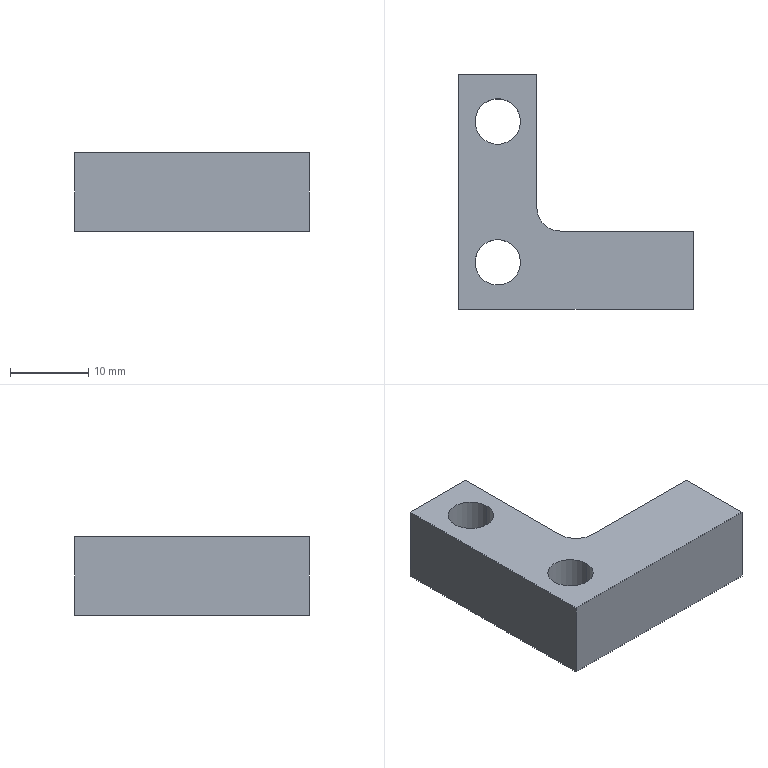Part | SolidWorks | features BaseBody 1 | 1 solid | 13 faces | box 30 x 30 x 10 mm | volume 4491 mm3 | plane 8 | cylinder 5 | commonest cylinder face diameters 5.8 x4 6 x1
STEP:
#1=CARTESIAN_POINT('',(-12.9,9.,0.));
#2=VERTEX_POINT('',#1);
#3=CARTESIAN_POINT('',(-12.9,9.,10.));
#4=VERTEX_POINT('',#3);
#5=CARTESIAN_POINT('',(-12.9,9.,10.));
#6=DIRECTION('',(0.,0.,1.));
#7=VECTOR('',#6,1000.);
#8=LINE('',#5,#7);
#9=EDGE_CURVE('',#2,#4,#8,.T.);
#10=ORIENTED_EDGE('',*,*,#9,.F.);
#11=CARTESIAN_POINT('',(-7.1,9.,0.));
#12=VERTEX_POINT('',#11);
#13=CARTESIAN_POINT('',(-10.,9.,0.));
#14=DIRECTION('',(0.,0.,1.));
#15=DIRECTION('',(1.,0.,0.));
#16=AXIS2_PLACEMENT_3D('',#13,#14,#15);
#17=CIRCLE('',#16,2.9);
#18=EDGE_CURVE('',#12,#2,#17,.T.);
#19=ORIENTED_EDGE('',*,*,#18,.F.);
#20=CARTESIAN_POINT('',(-7.1,9.,10.));
#21=VERTEX_POINT('',#20);
#22=CARTESIAN_POINT('',(-7.1,9.,10.));
#23=DIRECTION('',(0.,0.,1.));
#24=VECTOR('',#23,1000.);
#25=LINE('',#22,#24);
#26=EDGE_CURVE('',#12,#21,#25,.T.);
#27=ORIENTED_EDGE('',*,*,#26,.T.);
#28=CARTESIAN_POINT('',(-10.,9.,10.));
#29=DIRECTION('',(0.,0.,1.));
#30=DIRECTION('',(1.,0.,0.));
#31=AXIS2_PLACEMENT_3D('',#28,#29,#30);
#32=CIRCLE('',#31,2.9);
#33=EDGE_CURVE('',#21,#4,#32,.T.);
#34=ORIENTED_EDGE('',*,*,#33,.T.);
#35=EDGE_LOOP('',(#10,#19,#27,#34));
#36=FACE_OUTER_BOUND('',#35,.T.);
#37=CARTESIAN_POINT('',(-10.,9.,10.));
#38=DIRECTION('',(0.,0.,1.));
#39=DIRECTION('',(1.,0.,0.));
#40=AXIS2_PLACEMENT_3D('',#37,#38,#39);
#41=CYLINDRICAL_SURFACE('',#40,2.9);
#42=ADVANCED_FACE('',(#36),#41,.F.);
#43=CARTESIAN_POINT('',(-12.9,-9.,0.));
#44=VERTEX_POINT('',#43);
#45=CARTESIAN_POINT('',(-12.9,-9.,10.));
#46=VERTEX_POINT('',#45);
#47=CARTESIAN_POINT('',(-12.9,-9.,10.));
#48=DIRECTION('',(0.,0.,1.));
#49=VECTOR('',#48,1000.);
#50=LINE('',#47,#49);
#51=EDGE_CURVE('',#44,#46,#50,.T.);
#52=ORIENTED_EDGE('',*,*,#51,.F.);
#53=CARTESIAN_POINT('',(-7.1,-9.,0.));
#54=VERTEX_POINT('',#53);
#55=CARTESIAN_POINT('',(-10.,-9.,0.));
#56=DIRECTION('',(0.,0.,1.));
#57=DIRECTION('',(1.,0.,0.));
#58=AXIS2_PLACEMENT_3D('',#55,#56,#57);
#59=CIRCLE('',#58,2.9);
#60=EDGE_CURVE('',#54,#44,#59,.T.);
#61=ORIENTED_EDGE('',*,*,#60,.F.);
#62=CARTESIAN_POINT('',(-7.1,-9.,10.));
#63=VERTEX_POINT('',#62);
#64=CARTESIAN_POINT('',(-7.1,-9.,10.));
#65=DIRECTION('',(0.,0.,1.));
#66=VECTOR('',#65,1000.);
#67=LINE('',#64,#66);
#68=EDGE_CURVE('',#54,#63,#67,.T.);
#69=ORIENTED_EDGE('',*,*,#68,.T.);
#70=CARTESIAN_POINT('',(-10.,-9.,10.));
#71=DIRECTION('',(0.,0.,1.));
#72=DIRECTION('',(1.,0.,0.));
#73=AXIS2_PLACEMENT_3D('',#70,#71,#72);
#74=CIRCLE('',#73,2.9);
#75=EDGE_CURVE('',#63,#46,#74,.T.);
#76=ORIENTED_EDGE('',*,*,#75,.T.);
#77=EDGE_LOOP('',(#52,#61,#69,#76));
#78=FACE_OUTER_BOUND('',#77,.T.);
#79=CARTESIAN_POINT('',(-10.,-9.,10.));
#80=DIRECTION('',(0.,0.,1.));
#81=DIRECTION('',(1.,0.,0.));
#82=AXIS2_PLACEMENT_3D('',#79,#80,#81);
#83=CYLINDRICAL_SURFACE('',#82,2.9);
#84=ADVANCED_FACE('',(#78),#83,.F.);
#85=CARTESIAN_POINT('',(-5.,-2.,0.));
#86=VERTEX_POINT('',#85);
#87=CARTESIAN_POINT('',(-2.,-5.,0.));
#88=VERTEX_POINT('',#87);
#89=CARTESIAN_POINT('',(-2.,-2.,0.));
#90=DIRECTION('',(0.,0.,1.));
#91=DIRECTION('',(1.,0.,0.));
#92=AXIS2_PLACEMENT_3D('',#89,#90,#91);
#93=CIRCLE('',#92,3.);
#94=EDGE_CURVE('',#86,#88,#93,.T.);
#95=ORIENTED_EDGE('',*,*,#94,.F.);
#96=CARTESIAN_POINT('',(-5.,-2.,10.));
#97=VERTEX_POINT('',#96);
#98=CARTESIAN_POINT('',(-5.,-2.,0.));
#99=DIRECTION('',(0.,0.,-1.));
#100=VECTOR('',#99,1000.);
#101=LINE('',#98,#100);
#102=EDGE_CURVE('',#97,#86,#101,.T.);
#103=ORIENTED_EDGE('',*,*,#102,.F.);
#104=CARTESIAN_POINT('',(-2.,-5.,10.));
#105=VERTEX_POINT('',#104);
#106=CARTESIAN_POINT('',(-2.,-2.,10.));
#107=DIRECTION('',(0.,0.,-1.));
#108=DIRECTION('',(1.,0.,0.));
#109=AXIS2_PLACEMENT_3D('',#106,#107,#108);
#110=CIRCLE('',#109,3.);
#111=EDGE_CURVE('',#105,#97,#110,.T.);
#112=ORIENTED_EDGE('',*,*,#111,.F.);
#113=CARTESIAN_POINT('',(-2.,-5.,10.));
#114=DIRECTION('',(0.,0.,1.));
#115=VECTOR('',#114,1000.);
#116=LINE('',#113,#115);
#117=EDGE_CURVE('',#88,#105,#116,.T.);
#118=ORIENTED_EDGE('',*,*,#117,.F.);
#119=EDGE_LOOP('',(#95,#103,#112,#118));
#120=FACE_OUTER_BOUND('',#119,.T.);
#121=CARTESIAN_POINT('',(-2.,-2.,-0.001));
#122=DIRECTION('',(0.,0.,-1.));
#123=DIRECTION('',(-1.,0.,0.));
#124=AXIS2_PLACEMENT_3D('',#121,#122,#123);
#125=CYLINDRICAL_SURFACE('',#124,3.);
#126=ADVANCED_FACE('',(#120),#125,.F.);
#127=CARTESIAN_POINT('',(-5.,15.,10.));
#128=VERTEX_POINT('',#127);
#129=CARTESIAN_POINT('',(-5.,15.,10.));
#130=DIRECTION('',(0.,-1.,0.));
#131=VECTOR('',#130,1000.);
#132=LINE('',#129,#131);
#133=EDGE_CURVE('',#128,#97,#132,.T.);
#134=ORIENTED_EDGE('',*,*,#133,.T.);
#135=ORIENTED_EDGE('',*,*,#102,.T.);
#136=CARTESIAN_POINT('',(-5.,15.,0.));
#137=VERTEX_POINT('',#136);
#138=CARTESIAN_POINT('',(-5.,15.,0.));
#139=DIRECTION('',(0.,1.,0.));
#140=VECTOR('',#139,1000.);
#141=LINE('',#138,#140);
#142=EDGE_CURVE('',#86,#137,#141,.T.);
#143=ORIENTED_EDGE('',*,*,#142,.T.);
#144=CARTESIAN_POINT('',(-5.,15.,-0.001));
#145=DIRECTION('',(0.,0.,1.));
#146=VECTOR('',#145,1000.);
#147=LINE('',#144,#146);
#148=EDGE_CURVE('',#137,#128,#147,.T.);
#149=ORIENTED_EDGE('',*,*,#148,.T.);
#150=EDGE_LOOP('',(#134,#135,#143,#149));
#151=FACE_OUTER_BOUND('',#150,.T.);
#152=CARTESIAN_POINT('',(-5.,15.,-0.001));
#153=DIRECTION('',(-1.,0.,0.));
#154=DIRECTION('',(0.,1.,0.));
#155=AXIS2_PLACEMENT_3D('',#152,#153,#154);
#156=PLANE('',#155);
#157=ADVANCED_FACE('',(#151),#156,.F.);
#158=CARTESIAN_POINT('',(15.,-5.,0.));
#159=VERTEX_POINT('',#158);
#160=CARTESIAN_POINT('',(15.,-5.,0.));
#161=DIRECTION('',(-1.,0.,0.));
#162=VECTOR('',#161,1000.);
#163=LINE('',#160,#162);
#164=EDGE_CURVE('',#159,#88,#163,.T.);
#165=ORIENTED_EDGE('',*,*,#164,.T.);
#166=ORIENTED_EDGE('',*,*,#117,.T.);
#167=CARTESIAN_POINT('',(15.,-5.,10.));
#168=VERTEX_POINT('',#167);
#169=CARTESIAN_POINT('',(15.,-5.,10.));
#170=DIRECTION('',(1.,0.,0.));
#171=VECTOR('',#170,1000.);
#172=LINE('',#169,#171);
#173=EDGE_CURVE('',#105,#168,#172,.T.);
#174=ORIENTED_EDGE('',*,*,#173,.T.);
#175=CARTESIAN_POINT('',(15.,-5.,-0.001));
#176=DIRECTION('',(0.,0.,1.));
#177=VECTOR('',#176,1000.);
#178=LINE('',#175,#177);
#179=EDGE_CURVE('',#159,#168,#178,.T.);
#180=ORIENTED_EDGE('',*,*,#179,.F.);
#181=EDGE_LOOP('',(#165,#166,#174,#180));
#182=FACE_OUTER_BOUND('',#181,.T.);
#183=CARTESIAN_POINT('',(15.,-5.,-0.001));
#184=DIRECTION('',(0.,-1.,0.));
#185=DIRECTION('',(0.,0.,-1.));
#186=AXIS2_PLACEMENT_3D('',#183,#184,#185);
#187=PLANE('',#186);
#188=ADVANCED_FACE('',(#182),#187,.F.);
#189=ORIENTED_EDGE('',*,*,#60,.T.);
#190=CARTESIAN_POINT('',(-10.,-9.,0.));
#191=DIRECTION('',(0.,0.,1.));
#192=DIRECTION('',(1.,0.,0.));
#193=AXIS2_PLACEMENT_3D('',#190,#191,#192);
#194=CIRCLE('',#193,2.9);
#195=EDGE_CURVE('',#44,#54,#194,.T.);
#196=ORIENTED_EDGE('',*,*,#195,.T.);
#197=EDGE_LOOP('',(#189,#196));
#198=FACE_BOUND('',#197,.T.);
#199=ORIENTED_EDGE('',*,*,#18,.T.);
#200=CARTESIAN_POINT('',(-10.,9.,0.));
#201=DIRECTION('',(0.,0.,1.));
#202=DIRECTION('',(1.,0.,0.));
#203=AXIS2_PLACEMENT_3D('',#200,#201,#202);
#204=CIRCLE('',#203,2.9);
#205=EDGE_CURVE('',#2,#12,#204,.T.);
#206=ORIENTED_EDGE('',*,*,#205,.T.);
#207=EDGE_LOOP('',(#199,#206));
#208=FACE_BOUND('',#207,.T.);
#209=ORIENTED_EDGE('',*,*,#142,.F.);
#210=ORIENTED_EDGE('',*,*,#94,.T.);
#211=ORIENTED_EDGE('',*,*,#164,.F.);
#212=CARTESIAN_POINT('',(15.,-15.,0.));
#213=VERTEX_POINT('',#212);
#214=CARTESIAN_POINT('',(15.,-15.,0.));
#215=DIRECTION('',(0.,1.,0.));
#216=VECTOR('',#215,1000.);
#217=LINE('',#214,#216);
#218=EDGE_CURVE('',#213,#159,#217,.T.);
#219=ORIENTED_EDGE('',*,*,#218,.F.);
#220=CARTESIAN_POINT('',(-15.,-15.,0.));
#221=VERTEX_POINT('',#220);
#222=CARTESIAN_POINT('',(15.,-15.,0.));
#223=DIRECTION('',(1.,0.,0.));
#224=VECTOR('',#223,1000.);
#225=LINE('',#222,#224);
#226=EDGE_CURVE('',#221,#213,#225,.T.);
#227=ORIENTED_EDGE('',*,*,#226,.F.);
#228=CARTESIAN_POINT('',(-15.,15.,0.));
#229=VERTEX_POINT('',#228);
#230=CARTESIAN_POINT('',(-15.,-15.,0.));
#231=DIRECTION('',(0.,-1.,0.));
#232=VECTOR('',#231,1000.);
#233=LINE('',#230,#232);
#234=EDGE_CURVE('',#229,#221,#233,.T.);
#235=ORIENTED_EDGE('',*,*,#234,.F.);
#236=CARTESIAN_POINT('',(15.,15.,0.));
#237=DIRECTION('',(-1.,0.,0.));
#238=VECTOR('',#237,1000.);
#239=LINE('',#236,#238);
#240=EDGE_CURVE('',#137,#229,#239,.T.);
#241=ORIENTED_EDGE('',*,*,#240,.F.);
#242=EDGE_LOOP('',(#209,#210,#211,#219,#227,#235,#241));
#243=FACE_OUTER_BOUND('',#242,.T.);
#244=CARTESIAN_POINT('',(0.,0.,0.));
#245=DIRECTION('',(0.,0.,1.));
#246=DIRECTION('',(1.,0.,0.));
#247=AXIS2_PLACEMENT_3D('',#244,#245,#246);
#248=PLANE('',#247);
#249=ADVANCED_FACE('',(#198,#208,#243),#248,.F.);
#250=ORIENTED_EDGE('',*,*,#75,.F.);
#251=CARTESIAN_POINT('',(-10.,-9.,10.));
#252=DIRECTION('',(0.,0.,1.));
#253=DIRECTION('',(1.,0.,0.));
#254=AXIS2_PLACEMENT_3D('',#251,#252,#253);
#255=CIRCLE('',#254,2.9);
#256=EDGE_CURVE('',#46,#63,#255,.T.);
#257=ORIENTED_EDGE('',*,*,#256,.F.);
#258=EDGE_LOOP('',(#250,#257));
#259=FACE_BOUND('',#258,.T.);
#260=ORIENTED_EDGE('',*,*,#33,.F.);
#261=CARTESIAN_POINT('',(-10.,9.,10.));
#262=DIRECTION('',(0.,0.,1.));
#263=DIRECTION('',(1.,0.,0.));
#264=AXIS2_PLACEMENT_3D('',#261,#262,#263);
#265=CIRCLE('',#264,2.9);
#266=EDGE_CURVE('',#4,#21,#265,.T.);
#267=ORIENTED_EDGE('',*,*,#266,.F.);
#268=EDGE_LOOP('',(#260,#267));
#269=FACE_BOUND('',#268,.T.);
#270=ORIENTED_EDGE('',*,*,#173,.F.);
#271=ORIENTED_EDGE('',*,*,#111,.T.);
#272=ORIENTED_EDGE('',*,*,#133,.F.);
#273=CARTESIAN_POINT('',(-15.,15.,10.));
#274=VERTEX_POINT('',#273);
#275=CARTESIAN_POINT('',(15.,15.,10.));
#276=DIRECTION('',(-1.,0.,0.));
#277=VECTOR('',#276,1000.);
#278=LINE('',#275,#277);
#279=EDGE_CURVE('',#128,#274,#278,.T.);
#280=ORIENTED_EDGE('',*,*,#279,.T.);
#281=CARTESIAN_POINT('',(-15.,-15.,10.));
#282=VERTEX_POINT('',#281);
#283=CARTESIAN_POINT('',(-15.,-15.,10.));
#284=DIRECTION('',(0.,-1.,0.));
#285=VECTOR('',#284,1000.);
#286=LINE('',#283,#285);
#287=EDGE_CURVE('',#274,#282,#286,.T.);
#288=ORIENTED_EDGE('',*,*,#287,.T.);
#289=CARTESIAN_POINT('',(15.,-15.,10.));
#290=VERTEX_POINT('',#289);
#291=CARTESIAN_POINT('',(15.,-15.,10.));
#292=DIRECTION('',(1.,0.,0.));
#293=VECTOR('',#292,1000.);
#294=LINE('',#291,#293);
#295=EDGE_CURVE('',#282,#290,#294,.T.);
#296=ORIENTED_EDGE('',*,*,#295,.T.);
#297=CARTESIAN_POINT('',(15.,-15.,10.));
#298=DIRECTION('',(0.,1.,0.));
#299=VECTOR('',#298,1000.);
#300=LINE('',#297,#299);
#301=EDGE_CURVE('',#290,#168,#300,.T.);
#302=ORIENTED_EDGE('',*,*,#301,.T.);
#303=EDGE_LOOP('',(#270,#271,#272,#280,#288,#296,#302));
#304=FACE_OUTER_BOUND('',#303,.T.);
#305=CARTESIAN_POINT('',(0.,0.,10.));
#306=DIRECTION('',(0.,0.,1.));
#307=DIRECTION('',(1.,0.,0.));
#308=AXIS2_PLACEMENT_3D('',#305,#306,#307);
#309=PLANE('',#308);
#310=ADVANCED_FACE('',(#259,#269,#304),#309,.T.);
#311=ORIENTED_EDGE('',*,*,#279,.F.);
#312=ORIENTED_EDGE('',*,*,#148,.F.);
#313=ORIENTED_EDGE('',*,*,#240,.T.);
#314=CARTESIAN_POINT('',(-15.,15.,10.));
#315=DIRECTION('',(0.,0.,-1.));
#316=VECTOR('',#315,1000.);
#317=LINE('',#314,#316);
#318=EDGE_CURVE('',#274,#229,#317,.T.);
#319=ORIENTED_EDGE('',*,*,#318,.F.);
#320=EDGE_LOOP('',(#311,#312,#313,#319));
#321=FACE_OUTER_BOUND('',#320,.T.);
#322=CARTESIAN_POINT('',(15.,15.,10.));
#323=DIRECTION('',(0.,-1.,0.));
#324=DIRECTION('',(0.,0.,-1.));
#325=AXIS2_PLACEMENT_3D('',#322,#323,#324);
#326=PLANE('',#325);
#327=ADVANCED_FACE('',(#321),#326,.F.);
#328=ORIENTED_EDGE('',*,*,#218,.T.);
#329=ORIENTED_EDGE('',*,*,#179,.T.);
#330=ORIENTED_EDGE('',*,*,#301,.F.);
#331=CARTESIAN_POINT('',(15.,-15.,10.));
#332=DIRECTION('',(0.,0.,-1.));
#333=VECTOR('',#332,1000.);
#334=LINE('',#331,#333);
#335=EDGE_CURVE('',#290,#213,#334,.T.);
#336=ORIENTED_EDGE('',*,*,#335,.T.);
#337=EDGE_LOOP('',(#328,#329,#330,#336));
#338=FACE_OUTER_BOUND('',#337,.T.);
#339=CARTESIAN_POINT('',(15.,-15.,10.));
#340=DIRECTION('',(-1.,0.,0.));
#341=DIRECTION('',(0.,0.,1.));
#342=AXIS2_PLACEMENT_3D('',#339,#340,#341);
#343=PLANE('',#342);
#344=ADVANCED_FACE('',(#338),#343,.F.);
#345=ORIENTED_EDGE('',*,*,#226,.T.);
#346=ORIENTED_EDGE('',*,*,#335,.F.);
#347=ORIENTED_EDGE('',*,*,#295,.F.);
#348=CARTESIAN_POINT('',(-15.,-15.,10.));
#349=DIRECTION('',(0.,0.,-1.));
#350=VECTOR('',#349,1000.);
#351=LINE('',#348,#350);
#352=EDGE_CURVE('',#282,#221,#351,.T.);
#353=ORIENTED_EDGE('',*,*,#352,.T.);
#354=EDGE_LOOP('',(#345,#346,#347,#353));
#355=FACE_OUTER_BOUND('',#354,.T.);
#356=CARTESIAN_POINT('',(15.,-15.,10.));
#357=DIRECTION('',(0.,1.,0.));
#358=DIRECTION('',(1.,0.,0.));
#359=AXIS2_PLACEMENT_3D('',#356,#357,#358);
#360=PLANE('',#359);
#361=ADVANCED_FACE('',(#355),#360,.F.);
#362=ORIENTED_EDGE('',*,*,#234,.T.);
#363=ORIENTED_EDGE('',*,*,#352,.F.);
#364=ORIENTED_EDGE('',*,*,#287,.F.);
#365=ORIENTED_EDGE('',*,*,#318,.T.);
#366=EDGE_LOOP('',(#362,#363,#364,#365));
#367=FACE_OUTER_BOUND('',#366,.T.);
#368=CARTESIAN_POINT('',(-15.,-15.,10.));
#369=DIRECTION('',(1.,0.,0.));
#370=DIRECTION('',(0.,1.,0.));
#371=AXIS2_PLACEMENT_3D('',#368,#369,#370);
#372=PLANE('',#371);
#373=ADVANCED_FACE('',(#367),#372,.F.);
#374=ORIENTED_EDGE('',*,*,#195,.F.);
#375=ORIENTED_EDGE('',*,*,#51,.T.);
#376=ORIENTED_EDGE('',*,*,#256,.T.);
#377=ORIENTED_EDGE('',*,*,#68,.F.);
#378=EDGE_LOOP('',(#374,#375,#376,#377));
#379=FACE_OUTER_BOUND('',#378,.T.);
#380=CARTESIAN_POINT('',(-10.,-9.,10.));
#381=DIRECTION('',(0.,0.,1.));
#382=DIRECTION('',(1.,0.,0.));
#383=AXIS2_PLACEMENT_3D('',#380,#381,#382);
#384=CYLINDRICAL_SURFACE('',#383,2.9);
#385=ADVANCED_FACE('',(#379),#384,.F.);
#386=ORIENTED_EDGE('',*,*,#205,.F.);
#387=ORIENTED_EDGE('',*,*,#9,.T.);
#388=ORIENTED_EDGE('',*,*,#266,.T.);
#389=ORIENTED_EDGE('',*,*,#26,.F.);
#390=EDGE_LOOP('',(#386,#387,#388,#389));
#391=FACE_OUTER_BOUND('',#390,.T.);
#392=CARTESIAN_POINT('',(-10.,9.,10.));
#393=DIRECTION('',(0.,0.,1.));
#394=DIRECTION('',(1.,0.,0.));
#395=AXIS2_PLACEMENT_3D('',#392,#393,#394);
#396=CYLINDRICAL_SURFACE('',#395,2.9);
#397=ADVANCED_FACE('',(#391),#396,.F.);
#398=CLOSED_SHELL('',(#42,#84,#126,#157,#188,#249,#310,#327,#344,#361,#373,#385,#397));
#399=MANIFOLD_SOLID_BREP('',#398);
#400=CARTESIAN_POINT('',(0.,0.,0.));
#401=DIRECTION('',(0.,0.,1.));
#402=DIRECTION('',(1.,0.,0.));
#403=AXIS2_PLACEMENT_3D('',#400,#401,#402);
#404=(LENGTH_UNIT()NAMED_UNIT(*)SI_UNIT(.MILLI.,.METRE.));
#405=UNCERTAINTY_MEASURE_WITH_UNIT(LENGTH_MEASURE(0.00001),#404,'','');
#406=(NAMED_UNIT(*)PLANE_ANGLE_UNIT()SI_UNIT($,.RADIAN.));
#407=(NAMED_UNIT(*)SI_UNIT($,.STERADIAN.)SOLID_ANGLE_UNIT());
#408=(GEOMETRIC_REPRESENTATION_CONTEXT(3)GLOBAL_UNCERTAINTY_ASSIGNED_CONTEXT((#405))GLOBAL_UNIT_ASSIGNED_CONTEXT((#404,#406,#407))REPRESENTATION_CONTEXT('',''));
#409=ADVANCED_BREP_SHAPE_REPRESENTATION('',(#399,#403),#408);